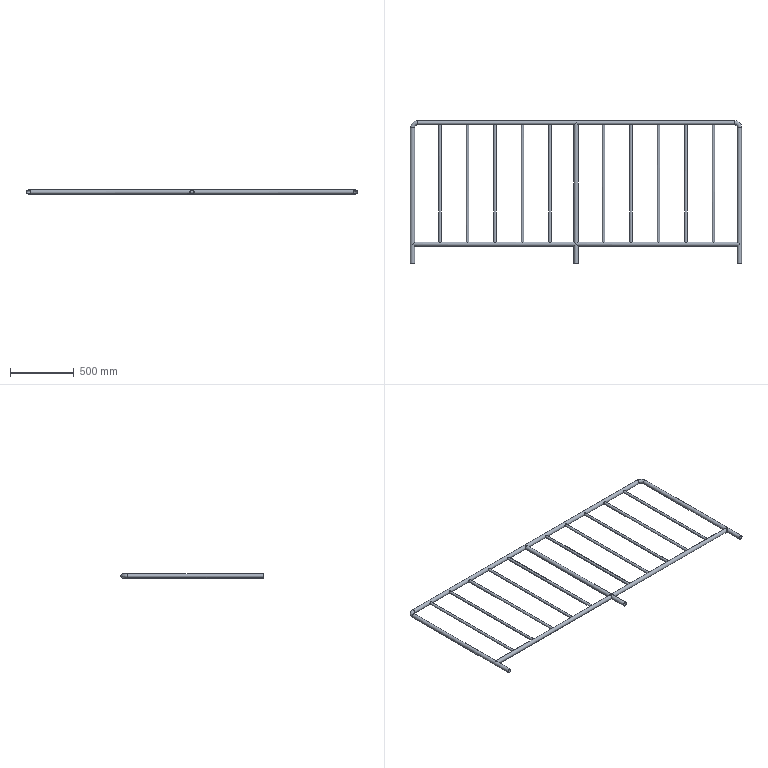Part | STEP file | PN_0058 304 guardrail 2560X1100 body-A_Default<As Machined> | 18 solids | 72 faces | box 2592 x 1116 x 32 mm | volume 2611653 mm3 | cylinder 57 | plane 11 | torus 4 | commonest cylinder face diameters 32 x31 16 x10 20 x10 28 x6